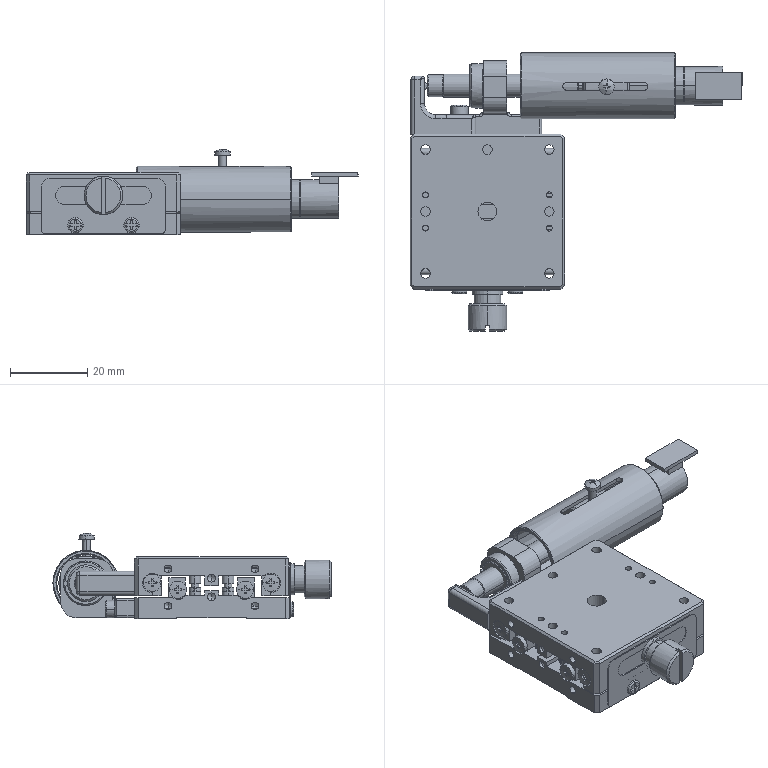Part | SolidWorks | 31 solids | 1283 faces | box 85.8 x 71.9 x 22.138 mm | volume 31070 mm3 | cylinder 485 | plane 455 | cone 259 | spline 48 | torus 36 | commonest cylinder face diameters 2.1 x89 2 x71 2.013 x58 3 x28 1.567 x24 4.5 x24